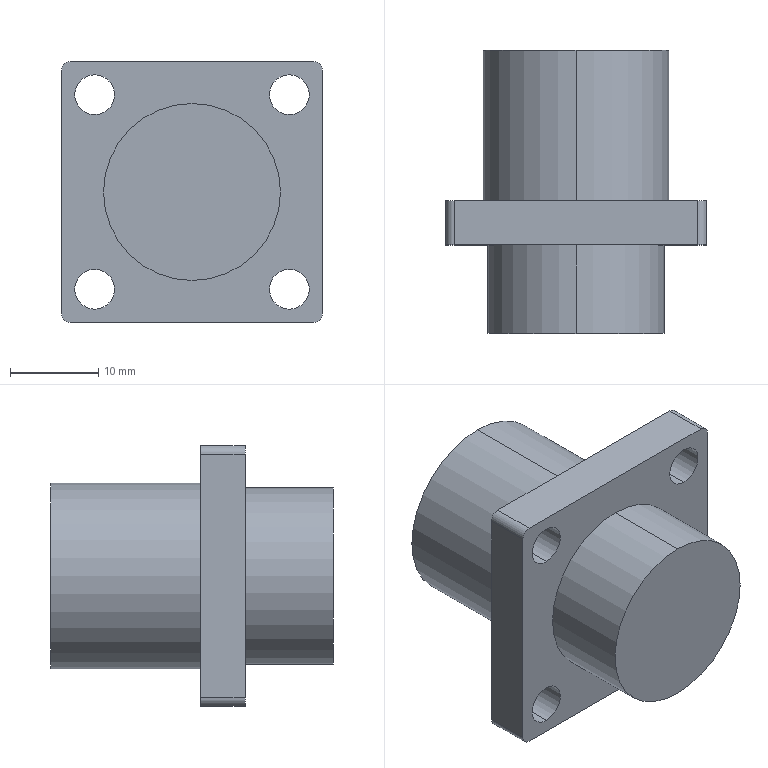Part | SolidWorks | features ICE 3, Extrusion 1, Fillet 1 | 1 solid | 24 faces | box 29.5 x 32 x 29.5 mm | volume 13059 mm3 | cylinder 16 | plane 8 | commonest cylinder face diameters 4.5 x8 2 x4 20 x2 21 x2
STEP:
#1=CARTESIAN_POINT('',(11.,10.,8.75));
#2=VERTEX_POINT('',#1);
#3=CARTESIAN_POINT('',(11.,10.,13.25));
#4=VERTEX_POINT('',#3);
#5=CARTESIAN_POINT('',(11.,10.,11.));
#6=DIRECTION('',(0.,1.,0.));
#7=DIRECTION('',(0.,0.,1.));
#8=AXIS2_PLACEMENT_3D('',#5,#6,#7);
#9=CIRCLE('',#8,2.25);
#10=EDGE_CURVE('',#2,#4,#9,.T.);
#11=ORIENTED_EDGE('',*,*,#10,.F.);
#12=CARTESIAN_POINT('',(11.,15.,8.75));
#13=VERTEX_POINT('',#12);
#14=CARTESIAN_POINT('',(11.,-2.,8.75));
#15=DIRECTION('',(0.,1.,0.));
#16=VECTOR('',#15,1000.);
#17=LINE('',#14,#16);
#18=EDGE_CURVE('',#2,#13,#17,.T.);
#19=ORIENTED_EDGE('',*,*,#18,.T.);
#20=CARTESIAN_POINT('',(11.,15.,13.25));
#21=VERTEX_POINT('',#20);
#22=CARTESIAN_POINT('',(11.,15.,11.));
#23=DIRECTION('',(0.,1.,0.));
#24=DIRECTION('',(0.,0.,1.));
#25=AXIS2_PLACEMENT_3D('',#22,#23,#24);
#26=CIRCLE('',#25,2.25);
#27=EDGE_CURVE('',#13,#21,#26,.T.);
#28=ORIENTED_EDGE('',*,*,#27,.T.);
#29=CARTESIAN_POINT('',(11.,-2.,13.25));
#30=DIRECTION('',(0.,1.,0.));
#31=VECTOR('',#30,1000.);
#32=LINE('',#29,#31);
#33=EDGE_CURVE('',#4,#21,#32,.T.);
#34=ORIENTED_EDGE('',*,*,#33,.F.);
#35=EDGE_LOOP('',(#11,#19,#28,#34));
#36=FACE_OUTER_BOUND('',#35,.T.);
#37=CARTESIAN_POINT('',(11.,-2.,11.));
#38=DIRECTION('',(0.,1.,0.));
#39=DIRECTION('',(0.,0.,1.));
#40=AXIS2_PLACEMENT_3D('',#37,#38,#39);
#41=CYLINDRICAL_SURFACE('',#40,2.25);
#42=ADVANCED_FACE('',(#36),#41,.F.);
#43=CARTESIAN_POINT('',(-11.,10.,8.75));
#44=VERTEX_POINT('',#43);
#45=CARTESIAN_POINT('',(-11.,10.,13.25));
#46=VERTEX_POINT('',#45);
#47=CARTESIAN_POINT('',(-11.,10.,11.));
#48=DIRECTION('',(0.,1.,0.));
#49=DIRECTION('',(0.,0.,1.));
#50=AXIS2_PLACEMENT_3D('',#47,#48,#49);
#51=CIRCLE('',#50,2.25);
#52=EDGE_CURVE('',#44,#46,#51,.T.);
#53=ORIENTED_EDGE('',*,*,#52,.F.);
#54=CARTESIAN_POINT('',(-11.,15.,8.75));
#55=VERTEX_POINT('',#54);
#56=CARTESIAN_POINT('',(-11.,-2.,8.75));
#57=DIRECTION('',(0.,1.,0.));
#58=VECTOR('',#57,1000.);
#59=LINE('',#56,#58);
#60=EDGE_CURVE('',#44,#55,#59,.T.);
#61=ORIENTED_EDGE('',*,*,#60,.T.);
#62=CARTESIAN_POINT('',(-11.,15.,13.25));
#63=VERTEX_POINT('',#62);
#64=CARTESIAN_POINT('',(-11.,15.,11.));
#65=DIRECTION('',(0.,1.,0.));
#66=DIRECTION('',(0.,0.,1.));
#67=AXIS2_PLACEMENT_3D('',#64,#65,#66);
#68=CIRCLE('',#67,2.25);
#69=EDGE_CURVE('',#55,#63,#68,.T.);
#70=ORIENTED_EDGE('',*,*,#69,.T.);
#71=CARTESIAN_POINT('',(-11.,-2.,13.25));
#72=DIRECTION('',(0.,1.,0.));
#73=VECTOR('',#72,1000.);
#74=LINE('',#71,#73);
#75=EDGE_CURVE('',#46,#63,#74,.T.);
#76=ORIENTED_EDGE('',*,*,#75,.F.);
#77=EDGE_LOOP('',(#53,#61,#70,#76));
#78=FACE_OUTER_BOUND('',#77,.T.);
#79=CARTESIAN_POINT('',(-11.,-2.,11.));
#80=DIRECTION('',(0.,1.,0.));
#81=DIRECTION('',(0.,0.,1.));
#82=AXIS2_PLACEMENT_3D('',#79,#80,#81);
#83=CYLINDRICAL_SURFACE('',#82,2.25);
#84=ADVANCED_FACE('',(#78),#83,.F.);
#85=CARTESIAN_POINT('',(-11.,10.,-13.25));
#86=VERTEX_POINT('',#85);
#87=CARTESIAN_POINT('',(-11.,10.,-8.75));
#88=VERTEX_POINT('',#87);
#89=CARTESIAN_POINT('',(-11.,10.,-11.));
#90=DIRECTION('',(0.,1.,0.));
#91=DIRECTION('',(0.,0.,1.));
#92=AXIS2_PLACEMENT_3D('',#89,#90,#91);
#93=CIRCLE('',#92,2.25);
#94=EDGE_CURVE('',#86,#88,#93,.T.);
#95=ORIENTED_EDGE('',*,*,#94,.F.);
#96=CARTESIAN_POINT('',(-11.,15.,-13.25));
#97=VERTEX_POINT('',#96);
#98=CARTESIAN_POINT('',(-11.,-2.,-13.25));
#99=DIRECTION('',(0.,1.,0.));
#100=VECTOR('',#99,1000.);
#101=LINE('',#98,#100);
#102=EDGE_CURVE('',#86,#97,#101,.T.);
#103=ORIENTED_EDGE('',*,*,#102,.T.);
#104=CARTESIAN_POINT('',(-11.,15.,-8.75));
#105=VERTEX_POINT('',#104);
#106=CARTESIAN_POINT('',(-11.,15.,-11.));
#107=DIRECTION('',(0.,1.,0.));
#108=DIRECTION('',(0.,0.,1.));
#109=AXIS2_PLACEMENT_3D('',#106,#107,#108);
#110=CIRCLE('',#109,2.25);
#111=EDGE_CURVE('',#97,#105,#110,.T.);
#112=ORIENTED_EDGE('',*,*,#111,.T.);
#113=CARTESIAN_POINT('',(-11.,-2.,-8.75));
#114=DIRECTION('',(0.,1.,0.));
#115=VECTOR('',#114,1000.);
#116=LINE('',#113,#115);
#117=EDGE_CURVE('',#88,#105,#116,.T.);
#118=ORIENTED_EDGE('',*,*,#117,.F.);
#119=EDGE_LOOP('',(#95,#103,#112,#118));
#120=FACE_OUTER_BOUND('',#119,.T.);
#121=CARTESIAN_POINT('',(-11.,-2.,-11.));
#122=DIRECTION('',(0.,1.,0.));
#123=DIRECTION('',(0.,0.,1.));
#124=AXIS2_PLACEMENT_3D('',#121,#122,#123);
#125=CYLINDRICAL_SURFACE('',#124,2.25);
#126=ADVANCED_FACE('',(#120),#125,.F.);
#127=CARTESIAN_POINT('',(11.,10.,-13.25));
#128=VERTEX_POINT('',#127);
#129=CARTESIAN_POINT('',(11.,10.,-8.75));
#130=VERTEX_POINT('',#129);
#131=CARTESIAN_POINT('',(11.,10.,-11.));
#132=DIRECTION('',(0.,1.,0.));
#133=DIRECTION('',(0.,0.,1.));
#134=AXIS2_PLACEMENT_3D('',#131,#132,#133);
#135=CIRCLE('',#134,2.25);
#136=EDGE_CURVE('',#128,#130,#135,.T.);
#137=ORIENTED_EDGE('',*,*,#136,.F.);
#138=CARTESIAN_POINT('',(11.,15.,-13.25));
#139=VERTEX_POINT('',#138);
#140=CARTESIAN_POINT('',(11.,-2.,-13.25));
#141=DIRECTION('',(0.,1.,0.));
#142=VECTOR('',#141,1000.);
#143=LINE('',#140,#142);
#144=EDGE_CURVE('',#128,#139,#143,.T.);
#145=ORIENTED_EDGE('',*,*,#144,.T.);
#146=CARTESIAN_POINT('',(11.,15.,-8.75));
#147=VERTEX_POINT('',#146);
#148=CARTESIAN_POINT('',(11.,15.,-11.));
#149=DIRECTION('',(0.,1.,0.));
#150=DIRECTION('',(0.,0.,1.));
#151=AXIS2_PLACEMENT_3D('',#148,#149,#150);
#152=CIRCLE('',#151,2.25);
#153=EDGE_CURVE('',#139,#147,#152,.T.);
#154=ORIENTED_EDGE('',*,*,#153,.T.);
#155=CARTESIAN_POINT('',(11.,-2.,-8.75));
#156=DIRECTION('',(0.,1.,0.));
#157=VECTOR('',#156,1000.);
#158=LINE('',#155,#157);
#159=EDGE_CURVE('',#130,#147,#158,.T.);
#160=ORIENTED_EDGE('',*,*,#159,.F.);
#161=EDGE_LOOP('',(#137,#145,#154,#160));
#162=FACE_OUTER_BOUND('',#161,.T.);
#163=CARTESIAN_POINT('',(11.,-2.,-11.));
#164=DIRECTION('',(0.,1.,0.));
#165=DIRECTION('',(0.,0.,1.));
#166=AXIS2_PLACEMENT_3D('',#163,#164,#165);
#167=CYLINDRICAL_SURFACE('',#166,2.25);
#168=ADVANCED_FACE('',(#162),#167,.F.);
#169=CARTESIAN_POINT('',(0.,32.,10.5));
#170=VERTEX_POINT('',#169);
#171=CARTESIAN_POINT('',(0.,32.,-10.5));
#172=VERTEX_POINT('',#171);
#173=CARTESIAN_POINT('',(0.,32.,0.));
#174=DIRECTION('',(0.,1.,0.));
#175=DIRECTION('',(0.,0.,1.));
#176=AXIS2_PLACEMENT_3D('',#173,#174,#175);
#177=CIRCLE('',#176,10.5);
#178=EDGE_CURVE('',#170,#172,#177,.T.);
#179=ORIENTED_EDGE('',*,*,#178,.F.);
#180=CARTESIAN_POINT('',(0.,15.,10.5));
#181=VERTEX_POINT('',#180);
#182=CARTESIAN_POINT('',(0.,32.,10.5));
#183=DIRECTION('',(0.,-1.,0.));
#184=VECTOR('',#183,1000.);
#185=LINE('',#182,#184);
#186=EDGE_CURVE('',#170,#181,#185,.T.);
#187=ORIENTED_EDGE('',*,*,#186,.T.);
#188=CARTESIAN_POINT('',(0.,15.,-10.5));
#189=VERTEX_POINT('',#188);
#190=CARTESIAN_POINT('',(0.,15.,0.));
#191=DIRECTION('',(0.,1.,0.));
#192=DIRECTION('',(0.,0.,1.));
#193=AXIS2_PLACEMENT_3D('',#190,#191,#192);
#194=CIRCLE('',#193,10.5);
#195=EDGE_CURVE('',#181,#189,#194,.T.);
#196=ORIENTED_EDGE('',*,*,#195,.T.);
#197=CARTESIAN_POINT('',(0.,32.,-10.5));
#198=DIRECTION('',(0.,-1.,0.));
#199=VECTOR('',#198,1000.);
#200=LINE('',#197,#199);
#201=EDGE_CURVE('',#172,#189,#200,.T.);
#202=ORIENTED_EDGE('',*,*,#201,.F.);
#203=EDGE_LOOP('',(#179,#187,#196,#202));
#204=FACE_OUTER_BOUND('',#203,.T.);
#205=CARTESIAN_POINT('',(0.,32.,0.));
#206=DIRECTION('',(0.,-1.,0.));
#207=DIRECTION('',(0.,0.,-1.));
#208=AXIS2_PLACEMENT_3D('',#205,#206,#207);
#209=CYLINDRICAL_SURFACE('',#208,10.5);
#210=ADVANCED_FACE('',(#204),#209,.T.);
#211=CARTESIAN_POINT('',(0.,10.,10.));
#212=VERTEX_POINT('',#211);
#213=CARTESIAN_POINT('',(0.,10.,-10.));
#214=VERTEX_POINT('',#213);
#215=CARTESIAN_POINT('',(0.,10.,0.));
#216=DIRECTION('',(0.,1.,0.));
#217=DIRECTION('',(0.,0.,1.));
#218=AXIS2_PLACEMENT_3D('',#215,#216,#217);
#219=CIRCLE('',#218,10.);
#220=EDGE_CURVE('',#212,#214,#219,.T.);
#221=ORIENTED_EDGE('',*,*,#220,.F.);
#222=CARTESIAN_POINT('',(0.,0.,10.));
#223=VERTEX_POINT('',#222);
#224=CARTESIAN_POINT('',(0.,10.,10.));
#225=DIRECTION('',(0.,-1.,0.));
#226=VECTOR('',#225,1000.);
#227=LINE('',#224,#226);
#228=EDGE_CURVE('',#212,#223,#227,.T.);
#229=ORIENTED_EDGE('',*,*,#228,.T.);
#230=CARTESIAN_POINT('',(0.,0.,-10.));
#231=VERTEX_POINT('',#230);
#232=CARTESIAN_POINT('',(0.,0.,0.));
#233=DIRECTION('',(0.,1.,0.));
#234=DIRECTION('',(0.,0.,1.));
#235=AXIS2_PLACEMENT_3D('',#232,#233,#234);
#236=CIRCLE('',#235,10.);
#237=EDGE_CURVE('',#223,#231,#236,.T.);
#238=ORIENTED_EDGE('',*,*,#237,.T.);
#239=CARTESIAN_POINT('',(0.,10.,-10.));
#240=DIRECTION('',(0.,-1.,0.));
#241=VECTOR('',#240,1000.);
#242=LINE('',#239,#241);
#243=EDGE_CURVE('',#214,#231,#242,.T.);
#244=ORIENTED_EDGE('',*,*,#243,.F.);
#245=EDGE_LOOP('',(#221,#229,#238,#244));
#246=FACE_OUTER_BOUND('',#245,.T.);
#247=CARTESIAN_POINT('',(0.,10.,0.));
#248=DIRECTION('',(0.,-1.,0.));
#249=DIRECTION('',(0.,0.,-1.));
#250=AXIS2_PLACEMENT_3D('',#247,#248,#249);
#251=CYLINDRICAL_SURFACE('',#250,10.);
#252=ADVANCED_FACE('',(#246),#251,.T.);
#253=CARTESIAN_POINT('',(11.,15.,11.));
#254=DIRECTION('',(0.,1.,0.));
#255=DIRECTION('',(0.,0.,1.));
#256=AXIS2_PLACEMENT_3D('',#253,#254,#255);
#257=CIRCLE('',#256,2.25);
#258=EDGE_CURVE('',#21,#13,#257,.T.);
#259=ORIENTED_EDGE('',*,*,#258,.F.);
#260=ORIENTED_EDGE('',*,*,#27,.F.);
#261=EDGE_LOOP('',(#259,#260));
#262=FACE_BOUND('',#261,.T.);
#263=CARTESIAN_POINT('',(-11.,15.,11.));
#264=DIRECTION('',(0.,1.,0.));
#265=DIRECTION('',(0.,0.,1.));
#266=AXIS2_PLACEMENT_3D('',#263,#264,#265);
#267=CIRCLE('',#266,2.25);
#268=EDGE_CURVE('',#63,#55,#267,.T.);
#269=ORIENTED_EDGE('',*,*,#268,.F.);
#270=ORIENTED_EDGE('',*,*,#69,.F.);
#271=EDGE_LOOP('',(#269,#270));
#272=FACE_BOUND('',#271,.T.);
#273=CARTESIAN_POINT('',(-11.,15.,-11.));
#274=DIRECTION('',(0.,1.,0.));
#275=DIRECTION('',(0.,0.,1.));
#276=AXIS2_PLACEMENT_3D('',#273,#274,#275);
#277=CIRCLE('',#276,2.25);
#278=EDGE_CURVE('',#105,#97,#277,.T.);
#279=ORIENTED_EDGE('',*,*,#278,.F.);
#280=ORIENTED_EDGE('',*,*,#111,.F.);
#281=EDGE_LOOP('',(#279,#280));
#282=FACE_BOUND('',#281,.T.);
#283=CARTESIAN_POINT('',(11.,15.,-11.));
#284=DIRECTION('',(0.,1.,0.));
#285=DIRECTION('',(0.,0.,1.));
#286=AXIS2_PLACEMENT_3D('',#283,#284,#285);
#287=CIRCLE('',#286,2.25);
#288=EDGE_CURVE('',#147,#139,#287,.T.);
#289=ORIENTED_EDGE('',*,*,#288,.F.);
#290=ORIENTED_EDGE('',*,*,#153,.F.);
#291=EDGE_LOOP('',(#289,#290));
#292=FACE_BOUND('',#291,.T.);
#293=CARTESIAN_POINT('',(13.75,15.,-14.75));
#294=VERTEX_POINT('',#293);
#295=CARTESIAN_POINT('',(-13.75,15.,-14.75));
#296=VERTEX_POINT('',#295);
#297=CARTESIAN_POINT('',(-14.75,15.,-14.75));
#298=DIRECTION('',(-1.,0.,0.));
#299=VECTOR('',#298,1000.);
#300=LINE('',#297,#299);
#301=EDGE_CURVE('',#294,#296,#300,.T.);
#302=ORIENTED_EDGE('',*,*,#301,.T.);
#303=CARTESIAN_POINT('',(-14.75,15.,-13.75));
#304=VERTEX_POINT('',#303);
#305=CARTESIAN_POINT('',(-13.75,15.,-13.75));
#306=DIRECTION('',(0.,1.,0.));
#307=DIRECTION('',(0.,0.,1.));
#308=AXIS2_PLACEMENT_3D('',#305,#306,#307);
#309=CIRCLE('',#308,1.);
#310=EDGE_CURVE('',#296,#304,#309,.T.);
#311=ORIENTED_EDGE('',*,*,#310,.T.);
#312=CARTESIAN_POINT('',(-14.75,15.,13.75));
#313=VERTEX_POINT('',#312);
#314=CARTESIAN_POINT('',(-14.75,15.,-14.75));
#315=DIRECTION('',(0.,0.,1.));
#316=VECTOR('',#315,1000.);
#317=LINE('',#314,#316);
#318=EDGE_CURVE('',#304,#313,#317,.T.);
#319=ORIENTED_EDGE('',*,*,#318,.T.);
#320=CARTESIAN_POINT('',(-13.75,15.,14.75));
#321=VERTEX_POINT('',#320);
#322=CARTESIAN_POINT('',(-13.75,15.,13.75));
#323=DIRECTION('',(0.,1.,0.));
#324=DIRECTION('',(0.,0.,1.));
#325=AXIS2_PLACEMENT_3D('',#322,#323,#324);
#326=CIRCLE('',#325,1.);
#327=EDGE_CURVE('',#313,#321,#326,.T.);
#328=ORIENTED_EDGE('',*,*,#327,.T.);
#329=CARTESIAN_POINT('',(13.75,15.,14.75));
#330=VERTEX_POINT('',#329);
#331=CARTESIAN_POINT('',(-14.75,15.,14.75));
#332=DIRECTION('',(1.,0.,0.));
#333=VECTOR('',#332,1000.);
#334=LINE('',#331,#333);
#335=EDGE_CURVE('',#321,#330,#334,.T.);
#336=ORIENTED_EDGE('',*,*,#335,.T.);
#337=CARTESIAN_POINT('',(14.75,15.,13.75));
#338=VERTEX_POINT('',#337);
#339=CARTESIAN_POINT('',(13.75,15.,13.75));
#340=DIRECTION('',(0.,1.,0.));
#341=DIRECTION('',(0.,0.,1.));
#342=AXIS2_PLACEMENT_3D('',#339,#340,#341);
#343=CIRCLE('',#342,1.);
#344=EDGE_CURVE('',#330,#338,#343,.T.);
#345=ORIENTED_EDGE('',*,*,#344,.T.);
#346=CARTESIAN_POINT('',(14.75,15.,-13.75));
#347=VERTEX_POINT('',#346);
#348=CARTESIAN_POINT('',(14.75,15.,-14.75));
#349=DIRECTION('',(0.,0.,-1.));
#350=VECTOR('',#349,1000.);
#351=LINE('',#348,#350);
#352=EDGE_CURVE('',#338,#347,#351,.T.);
#353=ORIENTED_EDGE('',*,*,#352,.T.);
#354=CARTESIAN_POINT('',(13.75,15.,-13.75));
#355=DIRECTION('',(0.,1.,0.));
#356=DIRECTION('',(0.,0.,1.));
#357=AXIS2_PLACEMENT_3D('',#354,#355,#356);
#358=CIRCLE('',#357,1.);
#359=EDGE_CURVE('',#347,#294,#358,.T.);
#360=ORIENTED_EDGE('',*,*,#359,.T.);
#361=EDGE_LOOP('',(#302,#311,#319,#328,#336,#345,#353,#360));
#362=FACE_OUTER_BOUND('',#361,.T.);
#363=CARTESIAN_POINT('',(0.,15.,0.));
#364=DIRECTION('',(0.,1.,0.));
#365=DIRECTION('',(0.,0.,1.));
#366=AXIS2_PLACEMENT_3D('',#363,#364,#365);
#367=CIRCLE('',#366,10.5);
#368=EDGE_CURVE('',#189,#181,#367,.T.);
#369=ORIENTED_EDGE('',*,*,#368,.F.);
#370=ORIENTED_EDGE('',*,*,#195,.F.);
#371=EDGE_LOOP('',(#369,#370));
#372=FACE_BOUND('',#371,.T.);
#373=CARTESIAN_POINT('',(0.,15.,0.));
#374=DIRECTION('',(0.,1.,0.));
#375=DIRECTION('',(0.,0.,1.));
#376=AXIS2_PLACEMENT_3D('',#373,#374,#375);
#377=PLANE('',#376);
#378=ADVANCED_FACE('',(#262,#272,#282,#292,#362,#372),#377,.T.);
#379=ORIENTED_EDGE('',*,*,#228,.F.);
#380=CARTESIAN_POINT('',(0.,10.,0.));
#381=DIRECTION('',(0.,1.,0.));
#382=DIRECTION('',(0.,0.,1.));
#383=AXIS2_PLACEMENT_3D('',#380,#381,#382);
#384=CIRCLE('',#383,10.);
#385=EDGE_CURVE('',#214,#212,#384,.T.);
#386=ORIENTED_EDGE('',*,*,#385,.F.);
#387=ORIENTED_EDGE('',*,*,#243,.T.);
#388=CARTESIAN_POINT('',(0.,0.,0.));
#389=DIRECTION('',(0.,1.,0.));
#390=DIRECTION('',(0.,0.,1.));
#391=AXIS2_PLACEMENT_3D('',#388,#389,#390);
#392=CIRCLE('',#391,10.);
#393=EDGE_CURVE('',#231,#223,#392,.T.);
#394=ORIENTED_EDGE('',*,*,#393,.T.);
#395=EDGE_LOOP('',(#379,#386,#387,#394));
#396=FACE_OUTER_BOUND('',#395,.T.);
#397=CARTESIAN_POINT('',(0.,10.,0.));
#398=DIRECTION('',(0.,-1.,0.));
#399=DIRECTION('',(0.,0.,-1.));
#400=AXIS2_PLACEMENT_3D('',#397,#398,#399);
#401=CYLINDRICAL_SURFACE('',#400,10.);
#402=ADVANCED_FACE('',(#396),#401,.T.);
#403=ORIENTED_EDGE('',*,*,#393,.F.);
#404=ORIENTED_EDGE('',*,*,#237,.F.);
#405=EDGE_LOOP('',(#403,#404));
#406=FACE_OUTER_BOUND('',#405,.T.);
#407=CARTESIAN_POINT('',(0.,0.,0.));
#408=DIRECTION('',(0.,1.,0.));
#409=DIRECTION('',(0.,0.,1.));
#410=AXIS2_PLACEMENT_3D('',#407,#408,#409);
#411=PLANE('',#410);
#412=ADVANCED_FACE('',(#406),#411,.F.);
#413=CARTESIAN_POINT('',(11.,10.,11.));
#414=DIRECTION('',(0.,1.,0.));
#415=DIRECTION('',(0.,0.,1.));
#416=AXIS2_PLACEMENT_3D('',#413,#414,#415);
#417=CIRCLE('',#416,2.25);
#418=EDGE_CURVE('',#4,#2,#417,.T.);
#419=ORIENTED_EDGE('',*,*,#418,.T.);
#420=ORIENTED_EDGE('',*,*,#10,.T.);
#421=EDGE_LOOP('',(#419,#420));
#422=FACE_BOUND('',#421,.T.);
#423=CARTESIAN_POINT('',(-11.,10.,11.));
#424=DIRECTION('',(0.,1.,0.));
#425=DIRECTION('',(0.,0.,1.));
#426=AXIS2_PLACEMENT_3D('',#423,#424,#425);
#427=CIRCLE('',#426,2.25);
#428=EDGE_CURVE('',#46,#44,#427,.T.);
#429=ORIENTED_EDGE('',*,*,#428,.T.);
#430=ORIENTED_EDGE('',*,*,#52,.T.);
#431=EDGE_LOOP('',(#429,#430));
#432=FACE_BOUND('',#431,.T.);
#433=CARTESIAN_POINT('',(-11.,10.,-11.));
#434=DIRECTION('',(0.,1.,0.));
#435=DIRECTION('',(0.,0.,1.));
#436=AXIS2_PLACEMENT_3D('',#433,#434,#435);
#437=CIRCLE('',#436,2.25);
#438=EDGE_CURVE('',#88,#86,#437,.T.);
#439=ORIENTED_EDGE('',*,*,#438,.T.);
#440=ORIENTED_EDGE('',*,*,#94,.T.);
#441=EDGE_LOOP('',(#439,#440));
#442=FACE_BOUND('',#441,.T.);
#443=CARTESIAN_POINT('',(11.,10.,-11.));
#444=DIRECTION('',(0.,1.,0.));
#445=DIRECTION('',(0.,0.,1.));
#446=AXIS2_PLACEMENT_3D('',#443,#444,#445);
#447=CIRCLE('',#446,2.25);
#448=EDGE_CURVE('',#130,#128,#447,.T.);
#449=ORIENTED_EDGE('',*,*,#448,.T.);
#450=ORIENTED_EDGE('',*,*,#136,.T.);
#451=EDGE_LOOP('',(#449,#450));
#452=FACE_BOUND('',#451,.T.);
#453=CARTESIAN_POINT('',(-14.75,10.,-13.75));
#454=VERTEX_POINT('',#453);
#455=CARTESIAN_POINT('',(-14.75,10.,13.75));
#456=VERTEX_POINT('',#455);
#457=CARTESIAN_POINT('',(-14.75,10.,-14.75));
#458=DIRECTION('',(0.,0.,1.));
#459=VECTOR('',#458,1000.);
#460=LINE('',#457,#459);
#461=EDGE_CURVE('',#454,#456,#460,.T.);
#462=ORIENTED_EDGE('',*,*,#461,.F.);
#463=CARTESIAN_POINT('',(-13.75,10.,-14.75));
#464=VERTEX_POINT('',#463);
#465=CARTESIAN_POINT('',(-13.75,10.,-13.75));
#466=DIRECTION('',(0.,-1.,0.));
#467=DIRECTION('',(0.,0.,1.));
#468=AXIS2_PLACEMENT_3D('',#465,#466,#467);
#469=CIRCLE('',#468,1.);
#470=EDGE_CURVE('',#454,#464,#469,.T.);
#471=ORIENTED_EDGE('',*,*,#470,.T.);
#472=CARTESIAN_POINT('',(13.75,10.,-14.75));
#473=VERTEX_POINT('',#472);
#474=CARTESIAN_POINT('',(-14.75,10.,-14.75));
#475=DIRECTION('',(-1.,0.,0.));
#476=VECTOR('',#475,1000.);
#477=LINE('',#474,#476);
#478=EDGE_CURVE('',#473,#464,#477,.T.);
#479=ORIENTED_EDGE('',*,*,#478,.F.);
#480=CARTESIAN_POINT('',(14.75,10.,-13.75));
#481=VERTEX_POINT('',#480);
#482=CARTESIAN_POINT('',(13.75,10.,-13.75));
#483=DIRECTION('',(0.,-1.,0.));
#484=DIRECTION('',(0.,0.,1.));
#485=AXIS2_PLACEMENT_3D('',#482,#483,#484);
#486=CIRCLE('',#485,1.);
#487=EDGE_CURVE('',#473,#481,#486,.T.);
#488=ORIENTED_EDGE('',*,*,#487,.T.);
#489=CARTESIAN_POINT('',(14.75,10.,13.75));
#490=VERTEX_POINT('',#489);
#491=CARTESIAN_POINT('',(14.75,10.,-14.75));
#492=DIRECTION('',(0.,0.,-1.));
#493=VECTOR('',#492,1000.);
#494=LINE('',#491,#493);
#495=EDGE_CURVE('',#490,#481,#494,.T.);
#496=ORIENTED_EDGE('',*,*,#495,.F.);
#497=CARTESIAN_POINT('',(13.75,10.,14.75));
#498=VERTEX_POINT('',#497);
#499=CARTESIAN_POINT('',(13.75,10.,13.75));
#500=DIRECTION('',(0.,-1.,0.));
#501=DIRECTION('',(0.,0.,1.));
#502=AXIS2_PLACEMENT_3D('',#499,#500,#501);
#503=CIRCLE('',#502,1.);
#504=EDGE_CURVE('',#490,#498,#503,.T.);
#505=ORIENTED_EDGE('',*,*,#504,.T.);
#506=CARTESIAN_POINT('',(-13.75,10.,14.75));
#507=VERTEX_POINT('',#506);
#508=CARTESIAN_POINT('',(-14.75,10.,14.75));
#509=DIRECTION('',(1.,0.,0.));
#510=VECTOR('',#509,1000.);
#511=LINE('',#508,#510);
#512=EDGE_CURVE('',#507,#498,#511,.T.);
#513=ORIENTED_EDGE('',*,*,#512,.F.);
#514=CARTESIAN_POINT('',(-13.75,10.,13.75));
#515=DIRECTION('',(0.,-1.,0.));
#516=DIRECTION('',(0.,0.,1.));
#517=AXIS2_PLACEMENT_3D('',#514,#515,#516);
#518=CIRCLE('',#517,1.);
#519=EDGE_CURVE('',#507,#456,#518,.T.);
#520=ORIENTED_EDGE('',*,*,#519,.T.);
#521=EDGE_LOOP('',(#462,#471,#479,#488,#496,#505,#513,#520));
#522=FACE_OUTER_BOUND('',#521,.T.);
#523=ORIENTED_EDGE('',*,*,#385,.T.);
#524=ORIENTED_EDGE('',*,*,#220,.T.);
#525=EDGE_LOOP('',(#523,#524));
#526=FACE_BOUND('',#525,.T.);
#527=CARTESIAN_POINT('',(0.,10.,0.));
#528=DIRECTION('',(0.,1.,0.));
#529=DIRECTION('',(0.,0.,1.));
#530=AXIS2_PLACEMENT_3D('',#527,#528,#529);
#531=PLANE('',#530);
#532=ADVANCED_FACE('',(#422,#432,#442,#452,#522,#526),#531,.F.);
#533=ORIENTED_EDGE('',*,*,#495,.T.);
#534=CARTESIAN_POINT('',(14.75,15.,-13.75));
#535=DIRECTION('',(0.,1.,0.));
#536=VECTOR('',#535,1000.);
#537=LINE('',#534,#536);
#538=EDGE_CURVE('',#481,#347,#537,.T.);
#539=ORIENTED_EDGE('',*,*,#538,.T.);
#540=ORIENTED_EDGE('',*,*,#352,.F.);
#541=CARTESIAN_POINT('',(14.75,15.,13.75));
#542=DIRECTION('',(0.,-1.,0.));
#543=VECTOR('',#542,1000.);
#544=LINE('',#541,#543);
#545=EDGE_CURVE('',#338,#490,#544,.T.);
#546=ORIENTED_EDGE('',*,*,#545,.T.);
#547=EDGE_LOOP('',(#533,#539,#540,#546));
#548=FACE_OUTER_BOUND('',#547,.T.);
#549=CARTESIAN_POINT('',(14.75,15.,-14.75));
#550=DIRECTION('',(-1.,0.,0.));
#551=DIRECTION('',(0.,0.,1.));
#552=AXIS2_PLACEMENT_3D('',#549,#550,#551);
#553=PLANE('',#552);
#554=ADVANCED_FACE('',(#548),#553,.F.);
#555=ORIENTED_EDGE('',*,*,#478,.T.);
#556=CARTESIAN_POINT('',(-13.75,15.,-14.75));
#557=DIRECTION('',(0.,1.,0.));
#558=VECTOR('',#557,1000.);
#559=LINE('',#556,#558);
#560=EDGE_CURVE('',#464,#296,#559,.T.);
#561=ORIENTED_EDGE('',*,*,#560,.T.);
#562=ORIENTED_EDGE('',*,*,#301,.F.);
#563=CARTESIAN_POINT('',(13.75,15.,-14.75));
#564=DIRECTION('',(0.,-1.,0.));
#565=VECTOR('',#564,1000.);
#566=LINE('',#563,#565);
#567=EDGE_CURVE('',#294,#473,#566,.T.);
#568=ORIENTED_EDGE('',*,*,#567,.T.);
#569=EDGE_LOOP('',(#555,#561,#562,#568));
#570=FACE_OUTER_BOUND('',#569,.T.);
#571=CARTESIAN_POINT('',(-14.75,15.,-14.75));
#572=DIRECTION('',(0.,0.,1.));
#573=DIRECTION('',(1.,0.,0.));
#574=AXIS2_PLACEMENT_3D('',#571,#572,#573);
#575=PLANE('',#574);
#576=ADVANCED_FACE('',(#570),#575,.F.);
#577=ORIENTED_EDGE('',*,*,#318,.F.);
#578=CARTESIAN_POINT('',(-14.75,15.,-13.75));
#579=DIRECTION('',(0.,-1.,0.));
#580=VECTOR('',#579,1000.);
#581=LINE('',#578,#580);
#582=EDGE_CURVE('',#304,#454,#581,.T.);
#583=ORIENTED_EDGE('',*,*,#582,.T.);
#584=ORIENTED_EDGE('',*,*,#461,.T.);
#585=CARTESIAN_POINT('',(-14.75,15.,13.75));
#586=DIRECTION('',(0.,1.,0.));
#587=VECTOR('',#586,1000.);
#588=LINE('',#585,#587);
#589=EDGE_CURVE('',#456,#313,#588,.T.);
#590=ORIENTED_EDGE('',*,*,#589,.T.);
#591=EDGE_LOOP('',(#577,#583,#584,#590));
#592=FACE_OUTER_BOUND('',#591,.T.);
#593=CARTESIAN_POINT('',(-14.75,15.,-14.75));
#594=DIRECTION('',(1.,0.,0.));
#595=DIRECTION('',(0.,0.,-1.));
#596=AXIS2_PLACEMENT_3D('',#593,#594,#595);
#597=PLANE('',#596);
#598=ADVANCED_FACE('',(#592),#597,.F.);
#599=ORIENTED_EDGE('',*,*,#512,.T.);
#600=CARTESIAN_POINT('',(13.75,15.,14.75));
#601=DIRECTION('',(0.,1.,0.));
#602=VECTOR('',#601,1000.);
#603=LINE('',#600,#602);
#604=EDGE_CURVE('',#498,#330,#603,.T.);
#605=ORIENTED_EDGE('',*,*,#604,.T.);
#606=ORIENTED_EDGE('',*,*,#335,.F.);
#607=CARTESIAN_POINT('',(-13.75,15.,14.75));
#608=DIRECTION('',(0.,-1.,0.));
#609=VECTOR('',#608,1000.);
#610=LINE('',#607,#609);
#611=EDGE_CURVE('',#321,#507,#610,.T.);
#612=ORIENTED_EDGE('',*,*,#611,.T.);
#613=EDGE_LOOP('',(#599,#605,#606,#612));
#614=FACE_OUTER_BOUND('',#613,.T.);
#615=CARTESIAN_POINT('',(-14.75,15.,14.75));
#616=DIRECTION('',(0.,0.,-1.));
#617=DIRECTION('',(-1.,0.,0.));
#618=AXIS2_PLACEMENT_3D('',#615,#616,#617);
#619=PLANE('',#618);
#620=ADVANCED_FACE('',(#614),#619,.F.);
#621=ORIENTED_EDGE('',*,*,#186,.F.);
#622=CARTESIAN_POINT('',(0.,32.,0.));
#623=DIRECTION('',(0.,1.,0.));
#624=DIRECTION('',(0.,0.,1.));
#625=AXIS2_PLACEMENT_3D('',#622,#623,#624);
#626=CIRCLE('',#625,10.5);
#627=EDGE_CURVE('',#172,#170,#626,.T.);
#628=ORIENTED_EDGE('',*,*,#627,.F.);
#629=ORIENTED_EDGE('',*,*,#201,.T.);
#630=ORIENTED_EDGE('',*,*,#368,.T.);
#631=EDGE_LOOP('',(#621,#628,#629,#630));
#632=FACE_OUTER_BOUND('',#631,.T.);
#633=CARTESIAN_POINT('',(0.,32.,0.));
#634=DIRECTION('',(0.,-1.,0.));
#635=DIRECTION('',(0.,0.,-1.));
#636=AXIS2_PLACEMENT_3D('',#633,#634,#635);
#637=CYLINDRICAL_SURFACE('',#636,10.5);
#638=ADVANCED_FACE('',(#632),#637,.T.);
#639=ORIENTED_EDGE('',*,*,#627,.T.);
#640=ORIENTED_EDGE('',*,*,#178,.T.);
#641=EDGE_LOOP('',(#639,#640));
#642=FACE_OUTER_BOUND('',#641,.T.);
#643=CARTESIAN_POINT('',(0.,32.,0.));
#644=DIRECTION('',(0.,1.,0.));
#645=DIRECTION('',(0.,0.,1.));
#646=AXIS2_PLACEMENT_3D('',#643,#644,#645);
#647=PLANE('',#646);
#648=ADVANCED_FACE('',(#642),#647,.T.);
#649=ORIENTED_EDGE('',*,*,#144,.F.);
#650=ORIENTED_EDGE('',*,*,#448,.F.);
#651=ORIENTED_EDGE('',*,*,#159,.T.);
#652=ORIENTED_EDGE('',*,*,#288,.T.);
#653=EDGE_LOOP('',(#649,#650,#651,#652));
#654=FACE_OUTER_BOUND('',#653,.T.);
#655=CARTESIAN_POINT('',(11.,-2.,-11.));
#656=DIRECTION('',(0.,1.,0.));
#657=DIRECTION('',(0.,0.,1.));
#658=AXIS2_PLACEMENT_3D('',#655,#656,#657);
#659=CYLINDRICAL_SURFACE('',#658,2.25);
#660=ADVANCED_FACE('',(#654),#659,.F.);
#661=ORIENTED_EDGE('',*,*,#102,.F.);
#662=ORIENTED_EDGE('',*,*,#438,.F.);
#663=ORIENTED_EDGE('',*,*,#117,.T.);
#664=ORIENTED_EDGE('',*,*,#278,.T.);
#665=EDGE_LOOP('',(#661,#662,#663,#664));
#666=FACE_OUTER_BOUND('',#665,.T.);
#667=CARTESIAN_POINT('',(-11.,-2.,-11.));
#668=DIRECTION('',(0.,1.,0.));
#669=DIRECTION('',(0.,0.,1.));
#670=AXIS2_PLACEMENT_3D('',#667,#668,#669);
#671=CYLINDRICAL_SURFACE('',#670,2.25);
#672=ADVANCED_FACE('',(#666),#671,.F.);
#673=ORIENTED_EDGE('',*,*,#60,.F.);
#674=ORIENTED_EDGE('',*,*,#428,.F.);
#675=ORIENTED_EDGE('',*,*,#75,.T.);
#676=ORIENTED_EDGE('',*,*,#268,.T.);
#677=EDGE_LOOP('',(#673,#674,#675,#676));
#678=FACE_OUTER_BOUND('',#677,.T.);
#679=CARTESIAN_POINT('',(-11.,-2.,11.));
#680=DIRECTION('',(0.,1.,0.));
#681=DIRECTION('',(0.,0.,1.));
#682=AXIS2_PLACEMENT_3D('',#679,#680,#681);
#683=CYLINDRICAL_SURFACE('',#682,2.25);
#684=ADVANCED_FACE('',(#678),#683,.F.);
#685=ORIENTED_EDGE('',*,*,#18,.F.);
#686=ORIENTED_EDGE('',*,*,#418,.F.);
#687=ORIENTED_EDGE('',*,*,#33,.T.);
#688=ORIENTED_EDGE('',*,*,#258,.T.);
#689=EDGE_LOOP('',(#685,#686,#687,#688));
#690=FACE_OUTER_BOUND('',#689,.T.);
#691=CARTESIAN_POINT('',(11.,-2.,11.));
#692=DIRECTION('',(0.,1.,0.));
#693=DIRECTION('',(0.,0.,1.));
#694=AXIS2_PLACEMENT_3D('',#691,#692,#693);
#695=CYLINDRICAL_SURFACE('',#694,2.25);
#696=ADVANCED_FACE('',(#690),#695,.F.);
#697=ORIENTED_EDGE('',*,*,#310,.F.);
#698=ORIENTED_EDGE('',*,*,#560,.F.);
#699=ORIENTED_EDGE('',*,*,#470,.F.);
#700=ORIENTED_EDGE('',*,*,#582,.F.);
#701=EDGE_LOOP('',(#697,#698,#699,#700));
#702=FACE_OUTER_BOUND('',#701,.T.);
#703=CARTESIAN_POINT('',(-13.75,15.,-13.75));
#704=DIRECTION('',(0.,-1.,0.));
#705=DIRECTION('',(0.,0.,-1.));
#706=AXIS2_PLACEMENT_3D('',#703,#704,#705);
#707=CYLINDRICAL_SURFACE('',#706,1.);
#708=ADVANCED_FACE('',(#702),#707,.T.);
#709=ORIENTED_EDGE('',*,*,#359,.F.);
#710=ORIENTED_EDGE('',*,*,#538,.F.);
#711=ORIENTED_EDGE('',*,*,#487,.F.);
#712=ORIENTED_EDGE('',*,*,#567,.F.);
#713=EDGE_LOOP('',(#709,#710,#711,#712));
#714=FACE_OUTER_BOUND('',#713,.T.);
#715=CARTESIAN_POINT('',(13.75,15.,-13.75));
#716=DIRECTION('',(0.,-1.,0.));
#717=DIRECTION('',(0.,0.,-1.));
#718=AXIS2_PLACEMENT_3D('',#715,#716,#717);
#719=CYLINDRICAL_SURFACE('',#718,1.);
#720=ADVANCED_FACE('',(#714),#719,.T.);
#721=ORIENTED_EDGE('',*,*,#344,.F.);
#722=ORIENTED_EDGE('',*,*,#604,.F.);
#723=ORIENTED_EDGE('',*,*,#504,.F.);
#724=ORIENTED_EDGE('',*,*,#545,.F.);
#725=EDGE_LOOP('',(#721,#722,#723,#724));
#726=FACE_OUTER_BOUND('',#725,.T.);
#727=CARTESIAN_POINT('',(13.75,15.,13.75));
#728=DIRECTION('',(0.,-1.,0.));
#729=DIRECTION('',(0.,0.,-1.));
#730=AXIS2_PLACEMENT_3D('',#727,#728,#729);
#731=CYLINDRICAL_SURFACE('',#730,1.);
#732=ADVANCED_FACE('',(#726),#731,.T.);
#733=ORIENTED_EDGE('',*,*,#327,.F.);
#734=ORIENTED_EDGE('',*,*,#589,.F.);
#735=ORIENTED_EDGE('',*,*,#519,.F.);
#736=ORIENTED_EDGE('',*,*,#611,.F.);
#737=EDGE_LOOP('',(#733,#734,#735,#736));
#738=FACE_OUTER_BOUND('',#737,.T.);
#739=CARTESIAN_POINT('',(-13.75,15.,13.75));
#740=DIRECTION('',(0.,-1.,0.));
#741=DIRECTION('',(0.,0.,-1.));
#742=AXIS2_PLACEMENT_3D('',#739,#740,#741);
#743=CYLINDRICAL_SURFACE('',#742,1.);
#744=ADVANCED_FACE('',(#738),#743,.T.);
#745=CLOSED_SHELL('',(#42,#84,#126,#168,#210,#252,#378,#402,#412,#532,#554,#576,#598,#620,#638,#648,#660,#672,#684,#696,#708,#720,#732,#744));
#746=MANIFOLD_SOLID_BREP('',#745);
#747=CARTESIAN_POINT('',(0.,0.,0.));
#748=DIRECTION('',(0.,0.,1.));
#749=DIRECTION('',(1.,0.,0.));
#750=AXIS2_PLACEMENT_3D('',#747,#748,#749);
#751=(LENGTH_UNIT()NAMED_UNIT(*)SI_UNIT(.MILLI.,.METRE.));
#752=UNCERTAINTY_MEASURE_WITH_UNIT(LENGTH_MEASURE(0.00001),#751,'','');
#753=(NAMED_UNIT(*)PLANE_ANGLE_UNIT()SI_UNIT($,.RADIAN.));
#754=(NAMED_UNIT(*)SI_UNIT($,.STERADIAN.)SOLID_ANGLE_UNIT());
#755=(GEOMETRIC_REPRESENTATION_CONTEXT(3)GLOBAL_UNCERTAINTY_ASSIGNED_CONTEXT((#752))GLOBAL_UNIT_ASSIGNED_CONTEXT((#751,#753,#754))REPRESENTATION_CONTEXT('',''));
#756=ADVANCED_BREP_SHAPE_REPRESENTATION('',(#746,#750),#755);